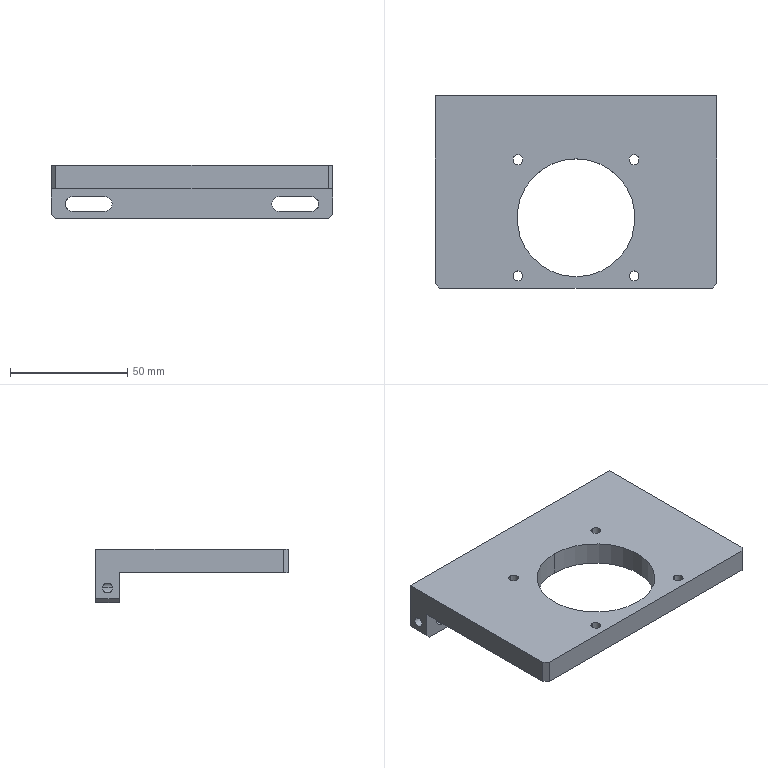NC program | NX | posted with a generic post | part box 120 x 82 x 22.8 mm
Lines 1 to 22 of 3479:
N10 G17 G21 G94 G90
(FLOOR_WALL , TOOL : D80)
N12 T19 M6
N14 G54
N16 G17 G0 G90 X-105. Y42.997 B0. C0. S6500 M3
N18 G43 Z30. H19
N20 Z3.
N22 G94 G1 Z0. F1500.
N24 X-102.
N26 X102.
N28 Y15.999
N30 X-102.
N32 Y-11.
N34 X102.
N36 X105.
N38 Z3.
N40 G0 Z30.
N42 M5